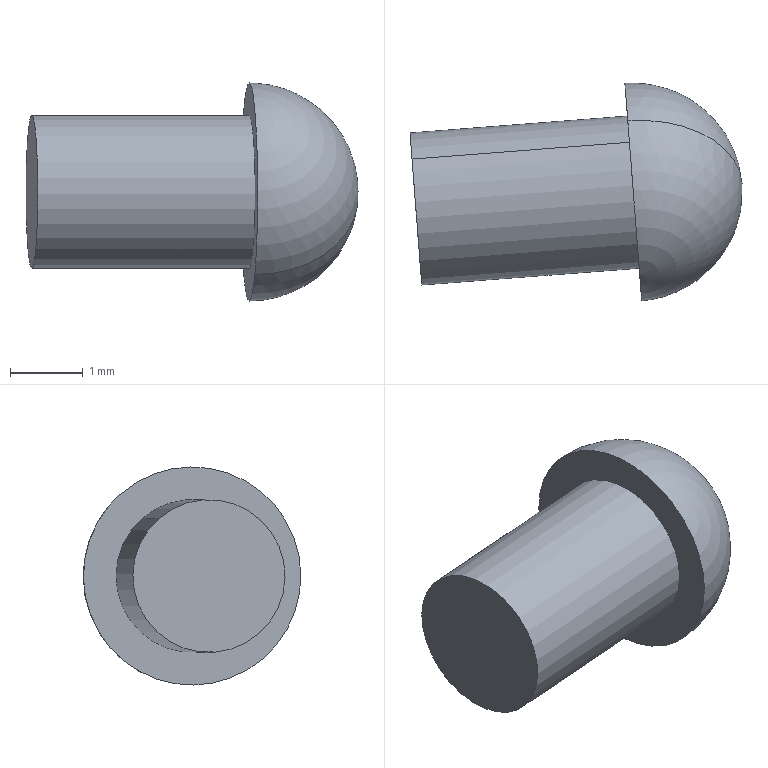Part | SolidWorks | features BaseBody 1 | 1 solid | 6 faces | box 4.572 x 2.996 x 3 mm | volume 17.459 mm3 | cylinder 2 | sphere 2 | plane 2 | commonest cylinder face diameters 2.1 x2
STEP:
#1=CARTESIAN_POINT('',(-23.749,83.92,2.044));
#2=VERTEX_POINT('',#1);
#3=CARTESIAN_POINT('',(-23.644,82.55,0.4559));
#4=VERTEX_POINT('',#3);
#5=CARTESIAN_POINT('',(-23.696,83.235,1.25));
#6=DIRECTION('',(-0.997,-0.07704,0.));
#7=DIRECTION('',(-0.05041,0.6523,0.7563));
#8=AXIS2_PLACEMENT_3D('',#5,#6,#7);
#9=CIRCLE('',#8,1.05);
#10=EDGE_CURVE('',#2,#4,#9,.T.);
#11=ORIENTED_EDGE('',*,*,#10,.F.);
#12=CARTESIAN_POINT('',(-20.758,84.151,2.044));
#13=VERTEX_POINT('',#12);
#14=CARTESIAN_POINT('',(-23.749,83.92,2.044));
#15=DIRECTION('',(0.997,0.07704,0.));
#16=VECTOR('',#15,1000.);
#17=LINE('',#14,#16);
#18=EDGE_CURVE('',#2,#13,#17,.T.);
#19=ORIENTED_EDGE('',*,*,#18,.T.);
#20=CARTESIAN_POINT('',(-20.652,82.781,0.4559));
#21=VERTEX_POINT('',#20);
#22=CARTESIAN_POINT('',(-20.705,83.466,1.25));
#23=DIRECTION('',(-0.997,-0.07704,0.));
#24=DIRECTION('',(-0.05041,0.6523,0.7563));
#25=AXIS2_PLACEMENT_3D('',#22,#23,#24);
#26=CIRCLE('',#25,1.05);
#27=EDGE_CURVE('',#13,#21,#26,.T.);
#28=ORIENTED_EDGE('',*,*,#27,.T.);
#29=CARTESIAN_POINT('',(-23.644,82.55,0.4559));
#30=DIRECTION('',(0.997,0.07704,0.));
#31=VECTOR('',#30,1000.);
#32=LINE('',#29,#31);
#33=EDGE_CURVE('',#4,#21,#32,.T.);
#34=ORIENTED_EDGE('',*,*,#33,.F.);
#35=EDGE_LOOP('',(#11,#19,#28,#34));
#36=FACE_OUTER_BOUND('',#35,.T.);
#37=CARTESIAN_POINT('',(-23.696,83.235,1.25));
#38=DIRECTION('',(0.997,0.07704,0.));
#39=DIRECTION('',(0.05041,-0.6523,-0.7563));
#40=AXIS2_PLACEMENT_3D('',#37,#38,#39);
#41=CYLINDRICAL_SURFACE('',#40,1.05);
#42=ADVANCED_FACE('',(#36),#41,.T.);
#43=CARTESIAN_POINT('',(-19.21,83.582,1.25));
#44=VERTEX_POINT('',#43);
#45=CARTESIAN_POINT('',(-20.781,84.444,2.384));
#46=VERTEX_POINT('',#45);
#47=CARTESIAN_POINT('',(-20.705,83.466,1.25));
#48=DIRECTION('',(0.05826,-0.754,0.6543));
#49=DIRECTION('',(0.,-0.6554,-0.7553));
#50=AXIS2_PLACEMENT_3D('',#47,#48,#49);
#51=CIRCLE('',#50,1.5);
#52=EDGE_CURVE('',#44,#46,#51,.T.);
#53=ORIENTED_EDGE('',*,*,#52,.F.);
#54=CARTESIAN_POINT('',(-20.63,82.487,0.1156));
#55=VERTEX_POINT('',#54);
#56=CARTESIAN_POINT('',(-20.705,83.466,1.25));
#57=DIRECTION('',(-0.05826,0.754,-0.6543));
#58=DIRECTION('',(0.,0.6554,0.7553));
#59=AXIS2_PLACEMENT_3D('',#56,#57,#58);
#60=CIRCLE('',#59,1.5);
#61=EDGE_CURVE('',#44,#55,#60,.T.);
#62=ORIENTED_EDGE('',*,*,#61,.T.);
#63=CARTESIAN_POINT('',(-20.705,83.466,1.25));
#64=DIRECTION('',(-0.997,-0.07704,0.));
#65=DIRECTION('',(-0.05041,0.6523,0.7563));
#66=AXIS2_PLACEMENT_3D('',#63,#64,#65);
#67=CIRCLE('',#66,1.5);
#68=EDGE_CURVE('',#46,#55,#67,.T.);
#69=ORIENTED_EDGE('',*,*,#68,.F.);
#70=EDGE_LOOP('',(#53,#62,#69));
#71=FACE_OUTER_BOUND('',#70,.T.);
#72=CARTESIAN_POINT('',(-20.705,83.466,1.25));
#73=DIRECTION('',(-0.05826,0.754,-0.6543));
#74=DIRECTION('',(-0.05041,0.6523,0.7563));
#75=AXIS2_PLACEMENT_3D('',#72,#73,#74);
#76=SPHERICAL_SURFACE('',#75,1.5);
#77=ADVANCED_FACE('',(#71),#76,.T.);
#78=ORIENTED_EDGE('',*,*,#61,.F.);
#79=ORIENTED_EDGE('',*,*,#52,.T.);
#80=CARTESIAN_POINT('',(-20.705,83.466,1.25));
#81=DIRECTION('',(-0.997,-0.07704,0.));
#82=DIRECTION('',(-0.05041,0.6523,0.7563));
#83=AXIS2_PLACEMENT_3D('',#80,#81,#82);
#84=CIRCLE('',#83,1.5);
#85=EDGE_CURVE('',#55,#46,#84,.T.);
#86=ORIENTED_EDGE('',*,*,#85,.F.);
#87=EDGE_LOOP('',(#78,#79,#86));
#88=FACE_OUTER_BOUND('',#87,.T.);
#89=CARTESIAN_POINT('',(-20.705,83.466,1.25));
#90=DIRECTION('',(-0.05826,0.754,-0.6543));
#91=DIRECTION('',(-0.05041,0.6523,0.7563));
#92=AXIS2_PLACEMENT_3D('',#89,#90,#91);
#93=SPHERICAL_SURFACE('',#92,1.5);
#94=ADVANCED_FACE('',(#88),#93,.T.);
#95=CARTESIAN_POINT('',(-20.705,83.466,1.25));
#96=DIRECTION('',(-0.997,-0.07704,0.));
#97=DIRECTION('',(-0.05041,0.6523,0.7563));
#98=AXIS2_PLACEMENT_3D('',#95,#96,#97);
#99=CIRCLE('',#98,1.05);
#100=EDGE_CURVE('',#21,#13,#99,.T.);
#101=ORIENTED_EDGE('',*,*,#100,.F.);
#102=ORIENTED_EDGE('',*,*,#27,.F.);
#103=EDGE_LOOP('',(#101,#102));
#104=FACE_BOUND('',#103,.T.);
#105=ORIENTED_EDGE('',*,*,#68,.T.);
#106=ORIENTED_EDGE('',*,*,#85,.T.);
#107=EDGE_LOOP('',(#105,#106));
#108=FACE_OUTER_BOUND('',#107,.T.);
#109=CARTESIAN_POINT('',(-20.705,83.466,1.25));
#110=DIRECTION('',(-0.997,-0.07704,0.));
#111=DIRECTION('',(-0.07704,0.997,0.));
#112=AXIS2_PLACEMENT_3D('',#109,#110,#111);
#113=PLANE('',#112);
#114=ADVANCED_FACE('',(#104,#108),#113,.T.);
#115=CARTESIAN_POINT('',(-23.696,83.235,1.25));
#116=DIRECTION('',(-0.997,-0.07704,0.));
#117=DIRECTION('',(-0.05041,0.6523,0.7563));
#118=AXIS2_PLACEMENT_3D('',#115,#116,#117);
#119=CIRCLE('',#118,1.05);
#120=EDGE_CURVE('',#4,#2,#119,.T.);
#121=ORIENTED_EDGE('',*,*,#120,.T.);
#122=ORIENTED_EDGE('',*,*,#10,.T.);
#123=EDGE_LOOP('',(#121,#122));
#124=FACE_OUTER_BOUND('',#123,.T.);
#125=CARTESIAN_POINT('',(-23.696,83.235,1.25));
#126=DIRECTION('',(-0.997,-0.07704,0.));
#127=DIRECTION('',(-0.07704,0.997,0.));
#128=AXIS2_PLACEMENT_3D('',#125,#126,#127);
#129=PLANE('',#128);
#130=ADVANCED_FACE('',(#124),#129,.T.);
#131=ORIENTED_EDGE('',*,*,#18,.F.);
#132=ORIENTED_EDGE('',*,*,#120,.F.);
#133=ORIENTED_EDGE('',*,*,#33,.T.);
#134=ORIENTED_EDGE('',*,*,#100,.T.);
#135=EDGE_LOOP('',(#131,#132,#133,#134));
#136=FACE_OUTER_BOUND('',#135,.T.);
#137=CARTESIAN_POINT('',(-23.696,83.235,1.25));
#138=DIRECTION('',(0.997,0.07704,0.));
#139=DIRECTION('',(0.05041,-0.6523,-0.7563));
#140=AXIS2_PLACEMENT_3D('',#137,#138,#139);
#141=CYLINDRICAL_SURFACE('',#140,1.05);
#142=ADVANCED_FACE('',(#136),#141,.T.);
#143=CLOSED_SHELL('',(#42,#77,#94,#114,#130,#142));
#144=MANIFOLD_SOLID_BREP('',#143);
#145=CARTESIAN_POINT('',(0.,0.,0.));
#146=DIRECTION('',(0.,0.,1.));
#147=DIRECTION('',(1.,0.,0.));
#148=AXIS2_PLACEMENT_3D('',#145,#146,#147);
#149=(LENGTH_UNIT()NAMED_UNIT(*)SI_UNIT(.MILLI.,.METRE.));
#150=UNCERTAINTY_MEASURE_WITH_UNIT(LENGTH_MEASURE(0.00001),#149,'','');
#151=(NAMED_UNIT(*)PLANE_ANGLE_UNIT()SI_UNIT($,.RADIAN.));
#152=(NAMED_UNIT(*)SI_UNIT($,.STERADIAN.)SOLID_ANGLE_UNIT());
#153=(GEOMETRIC_REPRESENTATION_CONTEXT(3)GLOBAL_UNCERTAINTY_ASSIGNED_CONTEXT((#150))GLOBAL_UNIT_ASSIGNED_CONTEXT((#149,#151,#152))REPRESENTATION_CONTEXT('',''));
#154=ADVANCED_BREP_SHAPE_REPRESENTATION('',(#144,#148),#153);